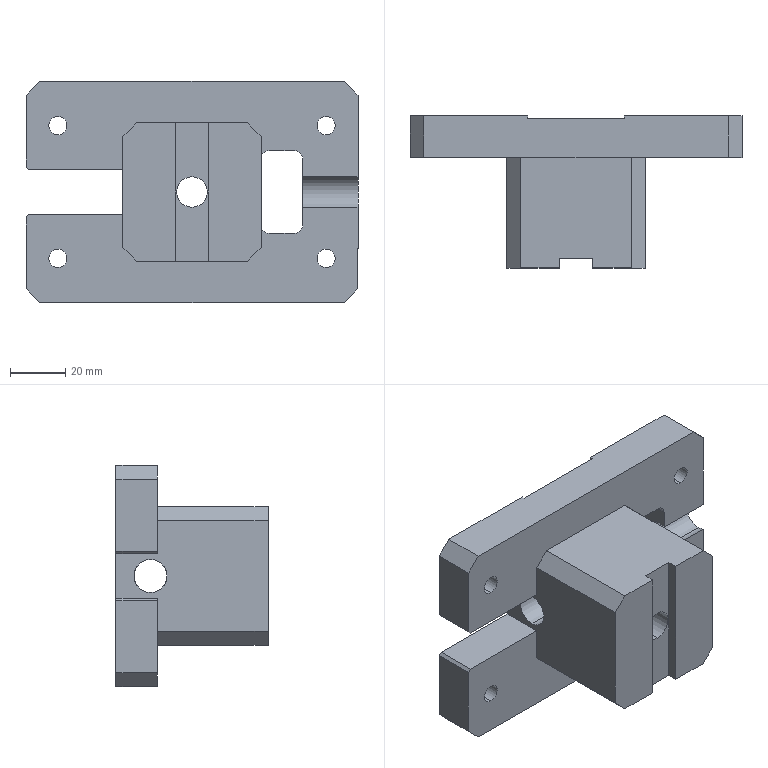Part | SolidWorks | features ICE 7, Chamfer 2, HoleWzd 2, Extrusion 1 | 1 solid | 86 faces | box 120 x 55 x 80 mm | volume 190025 mm3 | plane 49 | cylinder 37 | commonest cylinder face diameters 11 x10 6 x8 6.6 x8 12 x7 18 x4